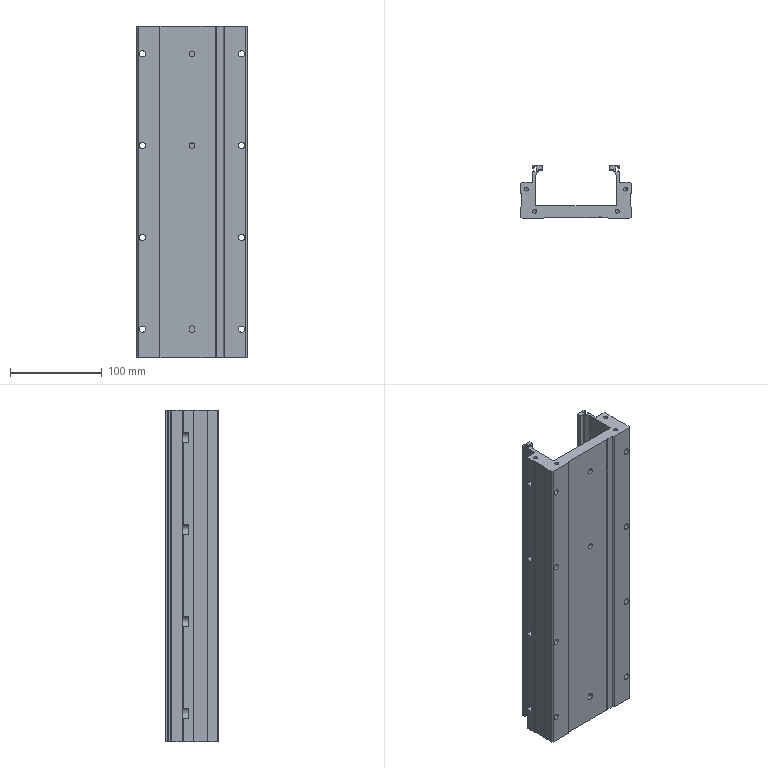Part | STEP file | LES120 base^FTH120-PD-direct-drive motor | 1 solid | 165 faces | box 120 x 58.2 x 361 mm | volume 888323 mm3 | plane 96 | cylinder 53 | cone 16 | commonest cylinder face diameters 4.2 x16 6.8 x16 11 x8 6 x6 1.2 x4 1 x2